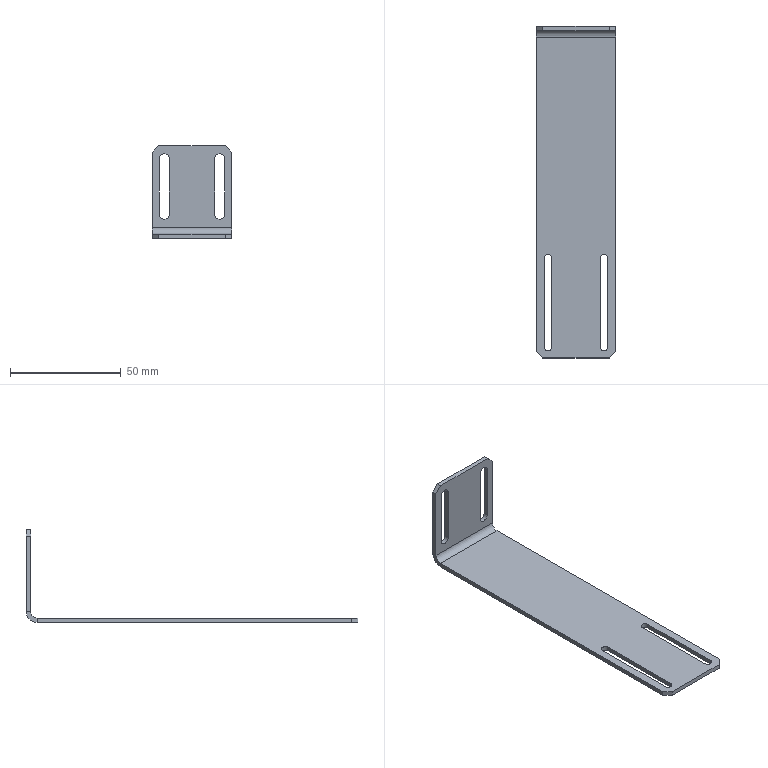Part | NX | 1 solid | 34 faces | box 36 x 150 x 42 mm | volume 12408 mm3 | plane 24 | cylinder 10 | commonest cylinder face diameters 3.5 x4 4.5 x4 6 x1 10 x1
STEP:
#1=CARTESIAN_POINT('',(-18.,70.,-2.));
#2=VERTEX_POINT('',#1);
#3=CARTESIAN_POINT('',(-18.,-72.,-2.));
#4=VERTEX_POINT('',#3);
#5=CARTESIAN_POINT('',(-18.,-75.,-2.));
#6=DIRECTION('',(0.,-1.,0.));
#7=VECTOR('',#6,1000.);
#8=LINE('',#5,#7);
#9=EDGE_CURVE('',#2,#4,#8,.T.);
#10=ORIENTED_EDGE('',*,*,#9,.T.);
#11=CARTESIAN_POINT('',(-18.,-72.,0.));
#12=VERTEX_POINT('',#11);
#13=CARTESIAN_POINT('',(-18.,-72.,-2.));
#14=DIRECTION('',(0.,0.,1.));
#15=VECTOR('',#14,1000.);
#16=LINE('',#13,#15);
#17=EDGE_CURVE('',#4,#12,#16,.T.);
#18=ORIENTED_EDGE('',*,*,#17,.T.);
#19=CARTESIAN_POINT('',(-18.,70.,0.));
#20=VERTEX_POINT('',#19);
#21=CARTESIAN_POINT('',(-18.,-75.,0.));
#22=DIRECTION('',(0.,-1.,0.));
#23=VECTOR('',#22,1000.);
#24=LINE('',#21,#23);
#25=EDGE_CURVE('',#20,#12,#24,.T.);
#26=ORIENTED_EDGE('',*,*,#25,.F.);
#27=CARTESIAN_POINT('',(-18.,70.,0.));
#28=DIRECTION('',(0.,0.,-1.));
#29=VECTOR('',#28,1000.);
#30=LINE('',#27,#29);
#31=EDGE_CURVE('',#20,#2,#30,.T.);
#32=ORIENTED_EDGE('',*,*,#31,.T.);
#33=EDGE_LOOP('',(#10,#18,#26,#32));
#34=FACE_BOUND('',#33,.T.);
#35=CARTESIAN_POINT('',(-18.,-75.,-2.));
#36=DIRECTION('',(-1.,0.,0.));
#37=DIRECTION('',(0.,0.,1.));
#38=AXIS2_PLACEMENT_3D('',#35,#36,#37);
#39=PLANE('',#38);
#40=ADVANCED_FACE('',(#34),#39,.T.);
#41=CARTESIAN_POINT('',(-14.45,-70.,-2.));
#42=VERTEX_POINT('',#41);
#43=CARTESIAN_POINT('',(-10.95,-70.,-2.));
#44=VERTEX_POINT('',#43);
#45=CARTESIAN_POINT('',(-12.7,-70.,-2.));
#46=DIRECTION('',(0.,0.,1.));
#47=DIRECTION('',(1.,0.,0.));
#48=AXIS2_PLACEMENT_3D('',#45,#46,#47);
#49=CIRCLE('',#48,1.75);
#50=EDGE_CURVE('',#42,#44,#49,.T.);
#51=ORIENTED_EDGE('',*,*,#50,.T.);
#52=CARTESIAN_POINT('',(-10.95,-30.,-2.));
#53=VERTEX_POINT('',#52);
#54=CARTESIAN_POINT('',(-10.95,-70.,-2.));
#55=DIRECTION('',(0.,1.,0.));
#56=VECTOR('',#55,1000.);
#57=LINE('',#54,#56);
#58=EDGE_CURVE('',#44,#53,#57,.T.);
#59=ORIENTED_EDGE('',*,*,#58,.T.);
#60=CARTESIAN_POINT('',(-14.45,-30.,-2.));
#61=VERTEX_POINT('',#60);
#62=CARTESIAN_POINT('',(-12.7,-30.,-2.));
#63=DIRECTION('',(0.,0.,1.));
#64=DIRECTION('',(1.,0.,0.));
#65=AXIS2_PLACEMENT_3D('',#62,#63,#64);
#66=CIRCLE('',#65,1.75);
#67=EDGE_CURVE('',#53,#61,#66,.T.);
#68=ORIENTED_EDGE('',*,*,#67,.T.);
#69=CARTESIAN_POINT('',(-14.45,-70.,-2.));
#70=DIRECTION('',(0.,-1.,0.));
#71=VECTOR('',#70,1000.);
#72=LINE('',#69,#71);
#73=EDGE_CURVE('',#61,#42,#72,.T.);
#74=ORIENTED_EDGE('',*,*,#73,.T.);
#75=EDGE_LOOP('',(#51,#59,#68,#74));
#76=FACE_BOUND('',#75,.T.);
#77=CARTESIAN_POINT('',(10.95,-70.,-2.));
#78=VERTEX_POINT('',#77);
#79=CARTESIAN_POINT('',(14.45,-70.,-2.));
#80=VERTEX_POINT('',#79);
#81=CARTESIAN_POINT('',(12.7,-70.,-2.));
#82=DIRECTION('',(0.,0.,1.));
#83=DIRECTION('',(1.,0.,0.));
#84=AXIS2_PLACEMENT_3D('',#81,#82,#83);
#85=CIRCLE('',#84,1.75);
#86=EDGE_CURVE('',#78,#80,#85,.T.);
#87=ORIENTED_EDGE('',*,*,#86,.T.);
#88=CARTESIAN_POINT('',(14.45,-30.,-2.));
#89=VERTEX_POINT('',#88);
#90=CARTESIAN_POINT('',(14.45,-70.,-2.));
#91=DIRECTION('',(0.,1.,0.));
#92=VECTOR('',#91,1000.);
#93=LINE('',#90,#92);
#94=EDGE_CURVE('',#80,#89,#93,.T.);
#95=ORIENTED_EDGE('',*,*,#94,.T.);
#96=CARTESIAN_POINT('',(10.95,-30.,-2.));
#97=VERTEX_POINT('',#96);
#98=CARTESIAN_POINT('',(12.7,-30.,-2.));
#99=DIRECTION('',(0.,0.,1.));
#100=DIRECTION('',(1.,0.,0.));
#101=AXIS2_PLACEMENT_3D('',#98,#99,#100);
#102=CIRCLE('',#101,1.75);
#103=EDGE_CURVE('',#89,#97,#102,.T.);
#104=ORIENTED_EDGE('',*,*,#103,.T.);
#105=CARTESIAN_POINT('',(10.95,-70.,-2.));
#106=DIRECTION('',(0.,-1.,0.));
#107=VECTOR('',#106,1000.);
#108=LINE('',#105,#107);
#109=EDGE_CURVE('',#97,#78,#108,.T.);
#110=ORIENTED_EDGE('',*,*,#109,.T.);
#111=EDGE_LOOP('',(#87,#95,#104,#110));
#112=FACE_BOUND('',#111,.T.);
#113=CARTESIAN_POINT('',(-15.,-75.,-2.));
#114=VERTEX_POINT('',#113);
#115=CARTESIAN_POINT('',(15.,-75.,-2.));
#116=VERTEX_POINT('',#115);
#117=CARTESIAN_POINT('',(-18.,-75.,-2.));
#118=DIRECTION('',(1.,0.,0.));
#119=VECTOR('',#118,1000.);
#120=LINE('',#117,#119);
#121=EDGE_CURVE('',#114,#116,#120,.T.);
#122=ORIENTED_EDGE('',*,*,#121,.F.);
#123=CARTESIAN_POINT('',(-45.,-45.,-2.));
#124=DIRECTION('',(0.7071,-0.7071,0.));
#125=VECTOR('',#124,1000.);
#126=LINE('',#123,#125);
#127=EDGE_CURVE('',#114,#4,#126,.F.);
#128=ORIENTED_EDGE('',*,*,#127,.T.);
#129=ORIENTED_EDGE('',*,*,#9,.F.);
#130=CARTESIAN_POINT('',(18.,70.,-2.));
#131=VERTEX_POINT('',#130);
#132=CARTESIAN_POINT('',(-18.,70.,-2.));
#133=DIRECTION('',(-1.,0.,0.));
#134=VECTOR('',#133,1000.);
#135=LINE('',#132,#134);
#136=EDGE_CURVE('',#2,#131,#135,.F.);
#137=ORIENTED_EDGE('',*,*,#136,.T.);
#138=CARTESIAN_POINT('',(18.,-72.,-2.));
#139=VERTEX_POINT('',#138);
#140=CARTESIAN_POINT('',(18.,-75.,-2.));
#141=DIRECTION('',(0.,1.,0.));
#142=VECTOR('',#141,1000.);
#143=LINE('',#140,#142);
#144=EDGE_CURVE('',#139,#131,#143,.T.);
#145=ORIENTED_EDGE('',*,*,#144,.F.);
#146=CARTESIAN_POINT('',(45.,-45.,-2.));
#147=DIRECTION('',(0.7071,0.7071,0.));
#148=VECTOR('',#147,1000.);
#149=LINE('',#146,#148);
#150=EDGE_CURVE('',#139,#116,#149,.F.);
#151=ORIENTED_EDGE('',*,*,#150,.T.);
#152=EDGE_LOOP('',(#122,#128,#129,#137,#145,#151));
#153=FACE_BOUND('',#152,.T.);
#154=CARTESIAN_POINT('',(0.,0.,-2.));
#155=DIRECTION('',(0.,0.,-1.));
#156=DIRECTION('',(-1.,0.,0.));
#157=AXIS2_PLACEMENT_3D('',#154,#155,#156);
#158=PLANE('',#157);
#159=ADVANCED_FACE('',(#76,#112,#153),#158,.T.);
#160=CARTESIAN_POINT('',(-10.95,-70.,0.));
#161=VERTEX_POINT('',#160);
#162=CARTESIAN_POINT('',(-10.95,-30.,0.));
#163=VERTEX_POINT('',#162);
#164=CARTESIAN_POINT('',(-10.95,-70.,0.));
#165=DIRECTION('',(0.,1.,0.));
#166=VECTOR('',#165,1000.);
#167=LINE('',#164,#166);
#168=EDGE_CURVE('',#161,#163,#167,.T.);
#169=ORIENTED_EDGE('',*,*,#168,.F.);
#170=CARTESIAN_POINT('',(-14.45,-70.,0.));
#171=VERTEX_POINT('',#170);
#172=CARTESIAN_POINT('',(-12.7,-70.,0.));
#173=DIRECTION('',(0.,0.,1.));
#174=DIRECTION('',(1.,0.,0.));
#175=AXIS2_PLACEMENT_3D('',#172,#173,#174);
#176=CIRCLE('',#175,1.75);
#177=EDGE_CURVE('',#171,#161,#176,.T.);
#178=ORIENTED_EDGE('',*,*,#177,.F.);
#179=CARTESIAN_POINT('',(-14.45,-30.,0.));
#180=VERTEX_POINT('',#179);
#181=CARTESIAN_POINT('',(-14.45,-70.,0.));
#182=DIRECTION('',(0.,-1.,0.));
#183=VECTOR('',#182,1000.);
#184=LINE('',#181,#183);
#185=EDGE_CURVE('',#180,#171,#184,.T.);
#186=ORIENTED_EDGE('',*,*,#185,.F.);
#187=CARTESIAN_POINT('',(-12.7,-30.,0.));
#188=DIRECTION('',(0.,0.,1.));
#189=DIRECTION('',(1.,0.,0.));
#190=AXIS2_PLACEMENT_3D('',#187,#188,#189);
#191=CIRCLE('',#190,1.75);
#192=EDGE_CURVE('',#163,#180,#191,.T.);
#193=ORIENTED_EDGE('',*,*,#192,.F.);
#194=EDGE_LOOP('',(#169,#178,#186,#193));
#195=FACE_BOUND('',#194,.T.);
#196=CARTESIAN_POINT('',(14.45,-70.,0.));
#197=VERTEX_POINT('',#196);
#198=CARTESIAN_POINT('',(14.45,-30.,0.));
#199=VERTEX_POINT('',#198);
#200=CARTESIAN_POINT('',(14.45,-70.,0.));
#201=DIRECTION('',(0.,1.,0.));
#202=VECTOR('',#201,1000.);
#203=LINE('',#200,#202);
#204=EDGE_CURVE('',#197,#199,#203,.T.);
#205=ORIENTED_EDGE('',*,*,#204,.F.);
#206=CARTESIAN_POINT('',(10.95,-70.,0.));
#207=VERTEX_POINT('',#206);
#208=CARTESIAN_POINT('',(12.7,-70.,0.));
#209=DIRECTION('',(0.,0.,1.));
#210=DIRECTION('',(1.,0.,0.));
#211=AXIS2_PLACEMENT_3D('',#208,#209,#210);
#212=CIRCLE('',#211,1.75);
#213=EDGE_CURVE('',#207,#197,#212,.T.);
#214=ORIENTED_EDGE('',*,*,#213,.F.);
#215=CARTESIAN_POINT('',(10.95,-30.,0.));
#216=VERTEX_POINT('',#215);
#217=CARTESIAN_POINT('',(10.95,-70.,0.));
#218=DIRECTION('',(0.,-1.,0.));
#219=VECTOR('',#218,1000.);
#220=LINE('',#217,#219);
#221=EDGE_CURVE('',#216,#207,#220,.T.);
#222=ORIENTED_EDGE('',*,*,#221,.F.);
#223=CARTESIAN_POINT('',(12.7,-30.,0.));
#224=DIRECTION('',(0.,0.,1.));
#225=DIRECTION('',(1.,0.,0.));
#226=AXIS2_PLACEMENT_3D('',#223,#224,#225);
#227=CIRCLE('',#226,1.75);
#228=EDGE_CURVE('',#199,#216,#227,.T.);
#229=ORIENTED_EDGE('',*,*,#228,.F.);
#230=EDGE_LOOP('',(#205,#214,#222,#229));
#231=FACE_BOUND('',#230,.T.);
#232=ORIENTED_EDGE('',*,*,#25,.T.);
#233=CARTESIAN_POINT('',(-15.,-75.,0.));
#234=VERTEX_POINT('',#233);
#235=CARTESIAN_POINT('',(-18.,-72.,0.));
#236=DIRECTION('',(-0.7071,0.7071,0.));
#237=VECTOR('',#236,1000.);
#238=LINE('',#235,#237);
#239=EDGE_CURVE('',#12,#234,#238,.F.);
#240=ORIENTED_EDGE('',*,*,#239,.T.);
#241=CARTESIAN_POINT('',(15.,-75.,0.));
#242=VERTEX_POINT('',#241);
#243=CARTESIAN_POINT('',(-18.,-75.,0.));
#244=DIRECTION('',(1.,0.,0.));
#245=VECTOR('',#244,1000.);
#246=LINE('',#243,#245);
#247=EDGE_CURVE('',#234,#242,#246,.T.);
#248=ORIENTED_EDGE('',*,*,#247,.T.);
#249=CARTESIAN_POINT('',(18.,-72.,0.));
#250=VERTEX_POINT('',#249);
#251=CARTESIAN_POINT('',(15.,-75.,0.));
#252=DIRECTION('',(-0.7071,-0.7071,0.));
#253=VECTOR('',#252,1000.);
#254=LINE('',#251,#253);
#255=EDGE_CURVE('',#242,#250,#254,.F.);
#256=ORIENTED_EDGE('',*,*,#255,.T.);
#257=CARTESIAN_POINT('',(18.,70.,0.));
#258=VERTEX_POINT('',#257);
#259=CARTESIAN_POINT('',(18.,-75.,0.));
#260=DIRECTION('',(0.,1.,0.));
#261=VECTOR('',#260,1000.);
#262=LINE('',#259,#261);
#263=EDGE_CURVE('',#250,#258,#262,.T.);
#264=ORIENTED_EDGE('',*,*,#263,.T.);
#265=CARTESIAN_POINT('',(-18.,70.,0.));
#266=DIRECTION('',(-1.,0.,0.));
#267=VECTOR('',#266,1000.);
#268=LINE('',#265,#267);
#269=EDGE_CURVE('',#20,#258,#268,.F.);
#270=ORIENTED_EDGE('',*,*,#269,.F.);
#271=EDGE_LOOP('',(#232,#240,#248,#256,#264,#270));
#272=FACE_BOUND('',#271,.T.);
#273=CARTESIAN_POINT('',(0.,0.,0.));
#274=DIRECTION('',(0.,0.,-1.));
#275=DIRECTION('',(-1.,0.,0.));
#276=AXIS2_PLACEMENT_3D('',#273,#274,#275);
#277=PLANE('',#276);
#278=ADVANCED_FACE('',(#195,#231,#272),#277,.F.);
#279=ORIENTED_EDGE('',*,*,#263,.F.);
#280=CARTESIAN_POINT('',(18.,-72.,-2.));
#281=DIRECTION('',(0.,0.,-1.));
#282=VECTOR('',#281,1000.);
#283=LINE('',#280,#282);
#284=EDGE_CURVE('',#250,#139,#283,.T.);
#285=ORIENTED_EDGE('',*,*,#284,.T.);
#286=ORIENTED_EDGE('',*,*,#144,.T.);
#287=CARTESIAN_POINT('',(18.,70.,0.));
#288=DIRECTION('',(0.,0.,-1.));
#289=VECTOR('',#288,1000.);
#290=LINE('',#287,#289);
#291=EDGE_CURVE('',#258,#131,#290,.T.);
#292=ORIENTED_EDGE('',*,*,#291,.F.);
#293=EDGE_LOOP('',(#279,#285,#286,#292));
#294=FACE_BOUND('',#293,.T.);
#295=CARTESIAN_POINT('',(18.,-75.,-2.));
#296=DIRECTION('',(1.,0.,0.));
#297=DIRECTION('',(0.,0.,-1.));
#298=AXIS2_PLACEMENT_3D('',#295,#296,#297);
#299=PLANE('',#298);
#300=ADVANCED_FACE('',(#294),#299,.T.);
#301=ORIENTED_EDGE('',*,*,#247,.F.);
#302=CARTESIAN_POINT('',(-15.,-75.,-2.));
#303=DIRECTION('',(0.,0.,-1.));
#304=VECTOR('',#303,1000.);
#305=LINE('',#302,#304);
#306=EDGE_CURVE('',#234,#114,#305,.T.);
#307=ORIENTED_EDGE('',*,*,#306,.T.);
#308=ORIENTED_EDGE('',*,*,#121,.T.);
#309=CARTESIAN_POINT('',(15.,-75.,-2.));
#310=DIRECTION('',(0.,0.,1.));
#311=VECTOR('',#310,1000.);
#312=LINE('',#309,#311);
#313=EDGE_CURVE('',#116,#242,#312,.T.);
#314=ORIENTED_EDGE('',*,*,#313,.T.);
#315=EDGE_LOOP('',(#301,#307,#308,#314));
#316=FACE_BOUND('',#315,.T.);
#317=CARTESIAN_POINT('',(-18.,-75.,-2.));
#318=DIRECTION('',(0.,-1.,0.));
#319=DIRECTION('',(0.,0.,-1.));
#320=AXIS2_PLACEMENT_3D('',#317,#318,#319);
#321=PLANE('',#320);
#322=ADVANCED_FACE('',(#316),#321,.T.);
#323=CARTESIAN_POINT('',(18.,73.,3.));
#324=VERTEX_POINT('',#323);
#325=CARTESIAN_POINT('',(18.,75.,3.));
#326=VERTEX_POINT('',#325);
#327=CARTESIAN_POINT('',(18.,75.,3.));
#328=DIRECTION('',(0.,-1.,0.));
#329=VECTOR('',#328,1000.);
#330=LINE('',#327,#329);
#331=EDGE_CURVE('',#324,#326,#330,.F.);
#332=ORIENTED_EDGE('',*,*,#331,.F.);
#333=CARTESIAN_POINT('',(18.,70.,3.));
#334=DIRECTION('',(-1.,0.,0.));
#335=DIRECTION('',(0.,0.,1.));
#336=AXIS2_PLACEMENT_3D('',#333,#334,#335);
#337=CIRCLE('',#336,3.);
#338=EDGE_CURVE('',#258,#324,#337,.F.);
#339=ORIENTED_EDGE('',*,*,#338,.F.);
#340=ORIENTED_EDGE('',*,*,#291,.T.);
#341=CARTESIAN_POINT('',(18.,70.,3.));
#342=DIRECTION('',(-1.,0.,0.));
#343=DIRECTION('',(0.,0.,1.));
#344=AXIS2_PLACEMENT_3D('',#341,#342,#343);
#345=CIRCLE('',#344,5.);
#346=EDGE_CURVE('',#131,#326,#345,.F.);
#347=ORIENTED_EDGE('',*,*,#346,.T.);
#348=EDGE_LOOP('',(#332,#339,#340,#347));
#349=FACE_BOUND('',#348,.T.);
#350=CARTESIAN_POINT('',(18.,70.,3.));
#351=DIRECTION('',(1.,0.,0.));
#352=DIRECTION('',(0.,0.,-1.));
#353=AXIS2_PLACEMENT_3D('',#350,#351,#352);
#354=PLANE('',#353);
#355=ADVANCED_FACE('',(#349),#354,.T.);
#356=CARTESIAN_POINT('',(-18.,73.,3.));
#357=VERTEX_POINT('',#356);
#358=CARTESIAN_POINT('',(-18.,70.,3.));
#359=DIRECTION('',(-1.,0.,0.));
#360=DIRECTION('',(0.,0.,1.));
#361=AXIS2_PLACEMENT_3D('',#358,#359,#360);
#362=CIRCLE('',#361,3.);
#363=EDGE_CURVE('',#357,#20,#362,.T.);
#364=ORIENTED_EDGE('',*,*,#363,.F.);
#365=CARTESIAN_POINT('',(-18.,75.,3.));
#366=VERTEX_POINT('',#365);
#367=CARTESIAN_POINT('',(-18.,73.,3.));
#368=DIRECTION('',(0.,-1.,0.));
#369=VECTOR('',#368,1000.);
#370=LINE('',#367,#369);
#371=EDGE_CURVE('',#357,#366,#370,.F.);
#372=ORIENTED_EDGE('',*,*,#371,.T.);
#373=CARTESIAN_POINT('',(-18.,70.,3.));
#374=DIRECTION('',(-1.,0.,0.));
#375=DIRECTION('',(0.,0.,1.));
#376=AXIS2_PLACEMENT_3D('',#373,#374,#375);
#377=CIRCLE('',#376,5.);
#378=EDGE_CURVE('',#366,#2,#377,.T.);
#379=ORIENTED_EDGE('',*,*,#378,.T.);
#380=ORIENTED_EDGE('',*,*,#31,.F.);
#381=EDGE_LOOP('',(#364,#372,#379,#380));
#382=FACE_BOUND('',#381,.T.);
#383=CARTESIAN_POINT('',(-18.,70.,3.));
#384=DIRECTION('',(1.,0.,0.));
#385=DIRECTION('',(0.,0.,-1.));
#386=AXIS2_PLACEMENT_3D('',#383,#384,#385);
#387=PLANE('',#386);
#388=ADVANCED_FACE('',(#382),#387,.F.);
#389=ORIENTED_EDGE('',*,*,#136,.F.);
#390=ORIENTED_EDGE('',*,*,#378,.F.);
#391=CARTESIAN_POINT('',(18.,75.,3.));
#392=DIRECTION('',(-1.,0.,0.));
#393=VECTOR('',#392,1000.);
#394=LINE('',#391,#393);
#395=EDGE_CURVE('',#366,#326,#394,.F.);
#396=ORIENTED_EDGE('',*,*,#395,.T.);
#397=ORIENTED_EDGE('',*,*,#346,.F.);
#398=EDGE_LOOP('',(#389,#390,#396,#397));
#399=FACE_BOUND('',#398,.T.);
#400=CARTESIAN_POINT('',(-18.,70.,3.));
#401=DIRECTION('',(-1.,0.,0.));
#402=DIRECTION('',(0.,1.,0.));
#403=AXIS2_PLACEMENT_3D('',#400,#401,#402);
#404=CYLINDRICAL_SURFACE('',#403,5.);
#405=ADVANCED_FACE('',(#399),#404,.T.);
#406=ORIENTED_EDGE('',*,*,#269,.T.);
#407=ORIENTED_EDGE('',*,*,#338,.T.);
#408=CARTESIAN_POINT('',(18.,73.,3.));
#409=DIRECTION('',(-1.,0.,0.));
#410=VECTOR('',#409,1000.);
#411=LINE('',#408,#410);
#412=EDGE_CURVE('',#324,#357,#411,.T.);
#413=ORIENTED_EDGE('',*,*,#412,.T.);
#414=ORIENTED_EDGE('',*,*,#363,.T.);
#415=EDGE_LOOP('',(#406,#407,#413,#414));
#416=FACE_BOUND('',#415,.T.);
#417=CARTESIAN_POINT('',(-18.,70.,3.));
#418=DIRECTION('',(-1.,0.,0.));
#419=DIRECTION('',(0.,1.,0.));
#420=AXIS2_PLACEMENT_3D('',#417,#418,#419);
#421=CYLINDRICAL_SURFACE('',#420,3.);
#422=ADVANCED_FACE('',(#416),#421,.F.);
#423=CARTESIAN_POINT('',(18.,75.,37.));
#424=VERTEX_POINT('',#423);
#425=CARTESIAN_POINT('',(18.,75.,0.));
#426=DIRECTION('',(0.,0.,-1.));
#427=VECTOR('',#426,1000.);
#428=LINE('',#425,#427);
#429=EDGE_CURVE('',#424,#326,#428,.T.);
#430=ORIENTED_EDGE('',*,*,#429,.F.);
#431=CARTESIAN_POINT('',(18.,73.,37.));
#432=VERTEX_POINT('',#431);
#433=CARTESIAN_POINT('',(18.,75.,37.));
#434=DIRECTION('',(0.,-1.,0.));
#435=VECTOR('',#434,1000.);
#436=LINE('',#433,#435);
#437=EDGE_CURVE('',#424,#432,#436,.T.);
#438=ORIENTED_EDGE('',*,*,#437,.T.);
#439=CARTESIAN_POINT('',(18.,73.,0.));
#440=DIRECTION('',(0.,0.,1.));
#441=VECTOR('',#440,1000.);
#442=LINE('',#439,#441);
#443=EDGE_CURVE('',#432,#324,#442,.F.);
#444=ORIENTED_EDGE('',*,*,#443,.T.);
#445=ORIENTED_EDGE('',*,*,#331,.T.);
#446=EDGE_LOOP('',(#430,#438,#444,#445));
#447=FACE_BOUND('',#446,.T.);
#448=CARTESIAN_POINT('',(18.,75.,0.));
#449=DIRECTION('',(-1.,0.,0.));
#450=DIRECTION('',(0.,0.,1.));
#451=AXIS2_PLACEMENT_3D('',#448,#449,#450);
#452=PLANE('',#451);
#453=ADVANCED_FACE('',(#447),#452,.F.);
#454=CARTESIAN_POINT('',(-18.,73.,37.));
#455=VERTEX_POINT('',#454);
#456=CARTESIAN_POINT('',(-18.,73.,40.));
#457=DIRECTION('',(0.,0.,-1.));
#458=VECTOR('',#457,1000.);
#459=LINE('',#456,#458);
#460=EDGE_CURVE('',#357,#455,#459,.F.);
#461=ORIENTED_EDGE('',*,*,#460,.T.);
#462=CARTESIAN_POINT('',(-18.,75.,37.));
#463=VERTEX_POINT('',#462);
#464=CARTESIAN_POINT('',(-18.,75.,37.));
#465=DIRECTION('',(0.,1.,0.));
#466=VECTOR('',#465,1000.);
#467=LINE('',#464,#466);
#468=EDGE_CURVE('',#455,#463,#467,.T.);
#469=ORIENTED_EDGE('',*,*,#468,.T.);
#470=CARTESIAN_POINT('',(-18.,75.,0.));
#471=DIRECTION('',(0.,0.,1.));
#472=VECTOR('',#471,1000.);
#473=LINE('',#470,#472);
#474=EDGE_CURVE('',#366,#463,#473,.T.);
#475=ORIENTED_EDGE('',*,*,#474,.F.);
#476=ORIENTED_EDGE('',*,*,#371,.F.);
#477=EDGE_LOOP('',(#461,#469,#475,#476));
#478=FACE_BOUND('',#477,.T.);
#479=CARTESIAN_POINT('',(-18.,75.,40.));
#480=DIRECTION('',(1.,0.,0.));
#481=DIRECTION('',(0.,0.,-1.));
#482=AXIS2_PLACEMENT_3D('',#479,#480,#481);
#483=PLANE('',#482);
#484=ADVANCED_FACE('',(#478),#483,.F.);
#485=CARTESIAN_POINT('',(14.75,75.,9.));
#486=VERTEX_POINT('',#485);
#487=CARTESIAN_POINT('',(14.75,75.,34.));
#488=VERTEX_POINT('',#487);
#489=CARTESIAN_POINT('',(14.75,75.,34.));
#490=DIRECTION('',(0.,0.,1.));
#491=VECTOR('',#490,1000.);
#492=LINE('',#489,#491);
#493=EDGE_CURVE('',#486,#488,#492,.T.);
#494=ORIENTED_EDGE('',*,*,#493,.T.);
#495=CARTESIAN_POINT('',(10.25,75.,34.));
#496=VERTEX_POINT('',#495);
#497=CARTESIAN_POINT('',(12.5,75.,34.));
#498=DIRECTION('',(0.,-1.,0.));
#499=DIRECTION('',(0.,0.,-1.));
#500=AXIS2_PLACEMENT_3D('',#497,#498,#499);
#501=CIRCLE('',#500,2.25);
#502=EDGE_CURVE('',#488,#496,#501,.T.);
#503=ORIENTED_EDGE('',*,*,#502,.T.);
#504=CARTESIAN_POINT('',(10.25,75.,9.));
#505=VERTEX_POINT('',#504);
#506=CARTESIAN_POINT('',(10.25,75.,34.));
#507=DIRECTION('',(0.,0.,-1.));
#508=VECTOR('',#507,1000.);
#509=LINE('',#506,#508);
#510=EDGE_CURVE('',#496,#505,#509,.T.);
#511=ORIENTED_EDGE('',*,*,#510,.T.);
#512=CARTESIAN_POINT('',(12.5,75.,9.));
#513=DIRECTION('',(0.,-1.,0.));
#514=DIRECTION('',(0.,0.,-1.));
#515=AXIS2_PLACEMENT_3D('',#512,#513,#514);
#516=CIRCLE('',#515,2.25);
#517=EDGE_CURVE('',#505,#486,#516,.T.);
#518=ORIENTED_EDGE('',*,*,#517,.T.);
#519=EDGE_LOOP('',(#494,#503,#511,#518));
#520=FACE_BOUND('',#519,.T.);
#521=CARTESIAN_POINT('',(-10.25,75.,9.));
#522=VERTEX_POINT('',#521);
#523=CARTESIAN_POINT('',(-10.25,75.,34.));
#524=VERTEX_POINT('',#523);
#525=CARTESIAN_POINT('',(-10.25,75.,34.));
#526=DIRECTION('',(0.,0.,1.));
#527=VECTOR('',#526,1000.);
#528=LINE('',#525,#527);
#529=EDGE_CURVE('',#522,#524,#528,.T.);
#530=ORIENTED_EDGE('',*,*,#529,.T.);
#531=CARTESIAN_POINT('',(-14.75,75.,34.));
#532=VERTEX_POINT('',#531);
#533=CARTESIAN_POINT('',(-12.5,75.,34.));
#534=DIRECTION('',(0.,-1.,0.));
#535=DIRECTION('',(0.,0.,-1.));
#536=AXIS2_PLACEMENT_3D('',#533,#534,#535);
#537=CIRCLE('',#536,2.25);
#538=EDGE_CURVE('',#524,#532,#537,.T.);
#539=ORIENTED_EDGE('',*,*,#538,.T.);
#540=CARTESIAN_POINT('',(-14.75,75.,9.));
#541=VERTEX_POINT('',#540);
#542=CARTESIAN_POINT('',(-14.75,75.,34.));
#543=DIRECTION('',(0.,0.,-1.));
#544=VECTOR('',#543,1000.);
#545=LINE('',#542,#544);
#546=EDGE_CURVE('',#532,#541,#545,.T.);
#547=ORIENTED_EDGE('',*,*,#546,.T.);
#548=CARTESIAN_POINT('',(-12.5,75.,9.));
#549=DIRECTION('',(0.,-1.,0.));
#550=DIRECTION('',(0.,0.,-1.));
#551=AXIS2_PLACEMENT_3D('',#548,#549,#550);
#552=CIRCLE('',#551,2.25);
#553=EDGE_CURVE('',#541,#522,#552,.T.);
#554=ORIENTED_EDGE('',*,*,#553,.T.);
#555=EDGE_LOOP('',(#530,#539,#547,#554));
#556=FACE_BOUND('',#555,.T.);
#557=CARTESIAN_POINT('',(-15.,75.,40.));
#558=VERTEX_POINT('',#557);
#559=CARTESIAN_POINT('',(15.,75.,40.));
#560=VERTEX_POINT('',#559);
#561=CARTESIAN_POINT('',(0.,75.,40.));
#562=DIRECTION('',(1.,0.,0.));
#563=VECTOR('',#562,1000.);
#564=LINE('',#561,#563);
#565=EDGE_CURVE('',#558,#560,#564,.T.);
#566=ORIENTED_EDGE('',*,*,#565,.T.);
#567=CARTESIAN_POINT('',(18.,75.,37.));
#568=DIRECTION('',(-0.7071,0.,0.7071));
#569=VECTOR('',#568,1000.);
#570=LINE('',#567,#569);
#571=EDGE_CURVE('',#560,#424,#570,.F.);
#572=ORIENTED_EDGE('',*,*,#571,.T.);
#573=ORIENTED_EDGE('',*,*,#429,.T.);
#574=ORIENTED_EDGE('',*,*,#395,.F.);
#575=ORIENTED_EDGE('',*,*,#474,.T.);
#576=CARTESIAN_POINT('',(-15.,75.,40.));
#577=DIRECTION('',(-0.7071,0.,-0.7071));
#578=VECTOR('',#577,1000.);
#579=LINE('',#576,#578);
#580=EDGE_CURVE('',#463,#558,#579,.F.);
#581=ORIENTED_EDGE('',*,*,#580,.T.);
#582=EDGE_LOOP('',(#566,#572,#573,#574,#575,#581));
#583=FACE_BOUND('',#582,.T.);
#584=CARTESIAN_POINT('',(0.,75.,0.));
#585=DIRECTION('',(0.,-1.,0.));
#586=DIRECTION('',(0.,0.,-1.));
#587=AXIS2_PLACEMENT_3D('',#584,#585,#586);
#588=PLANE('',#587);
#589=ADVANCED_FACE('',(#520,#556,#583),#588,.F.);
#590=CARTESIAN_POINT('',(14.75,73.,34.));
#591=VERTEX_POINT('',#590);
#592=CARTESIAN_POINT('',(10.25,73.,34.));
#593=VERTEX_POINT('',#592);
#594=CARTESIAN_POINT('',(12.5,73.,34.));
#595=DIRECTION('',(0.,-1.,0.));
#596=DIRECTION('',(0.,0.,-1.));
#597=AXIS2_PLACEMENT_3D('',#594,#595,#596);
#598=CIRCLE('',#597,2.25);
#599=EDGE_CURVE('',#591,#593,#598,.T.);
#600=ORIENTED_EDGE('',*,*,#599,.F.);
#601=CARTESIAN_POINT('',(14.75,73.,9.));
#602=VERTEX_POINT('',#601);
#603=CARTESIAN_POINT('',(14.75,73.,34.));
#604=DIRECTION('',(0.,0.,1.));
#605=VECTOR('',#604,1000.);
#606=LINE('',#603,#605);
#607=EDGE_CURVE('',#602,#591,#606,.T.);
#608=ORIENTED_EDGE('',*,*,#607,.F.);
#609=CARTESIAN_POINT('',(10.25,73.,9.));
#610=VERTEX_POINT('',#609);
#611=CARTESIAN_POINT('',(12.5,73.,9.));
#612=DIRECTION('',(0.,-1.,0.));
#613=DIRECTION('',(0.,0.,-1.));
#614=AXIS2_PLACEMENT_3D('',#611,#612,#613);
#615=CIRCLE('',#614,2.25);
#616=EDGE_CURVE('',#610,#602,#615,.T.);
#617=ORIENTED_EDGE('',*,*,#616,.F.);
#618=CARTESIAN_POINT('',(10.25,73.,34.));
#619=DIRECTION('',(0.,0.,-1.));
#620=VECTOR('',#619,1000.);
#621=LINE('',#618,#620);
#622=EDGE_CURVE('',#593,#610,#621,.T.);
#623=ORIENTED_EDGE('',*,*,#622,.F.);
#624=EDGE_LOOP('',(#600,#608,#617,#623));
#625=FACE_BOUND('',#624,.T.);
#626=CARTESIAN_POINT('',(-10.25,73.,34.));
#627=VERTEX_POINT('',#626);
#628=CARTESIAN_POINT('',(-14.75,73.,34.));
#629=VERTEX_POINT('',#628);
#630=CARTESIAN_POINT('',(-12.5,73.,34.));
#631=DIRECTION('',(0.,-1.,0.));
#632=DIRECTION('',(0.,0.,-1.));
#633=AXIS2_PLACEMENT_3D('',#630,#631,#632);
#634=CIRCLE('',#633,2.25);
#635=EDGE_CURVE('',#627,#629,#634,.T.);
#636=ORIENTED_EDGE('',*,*,#635,.F.);
#637=CARTESIAN_POINT('',(-10.25,73.,9.));
#638=VERTEX_POINT('',#637);
#639=CARTESIAN_POINT('',(-10.25,73.,34.));
#640=DIRECTION('',(0.,0.,1.));
#641=VECTOR('',#640,1000.);
#642=LINE('',#639,#641);
#643=EDGE_CURVE('',#638,#627,#642,.T.);
#644=ORIENTED_EDGE('',*,*,#643,.F.);
#645=CARTESIAN_POINT('',(-14.75,73.,9.));
#646=VERTEX_POINT('',#645);
#647=CARTESIAN_POINT('',(-12.5,73.,9.));
#648=DIRECTION('',(0.,-1.,0.));
#649=DIRECTION('',(0.,0.,-1.));
#650=AXIS2_PLACEMENT_3D('',#647,#648,#649);
#651=CIRCLE('',#650,2.25);
#652=EDGE_CURVE('',#646,#638,#651,.T.);
#653=ORIENTED_EDGE('',*,*,#652,.F.);
#654=CARTESIAN_POINT('',(-14.75,73.,34.));
#655=DIRECTION('',(0.,0.,-1.));
#656=VECTOR('',#655,1000.);
#657=LINE('',#654,#656);
#658=EDGE_CURVE('',#629,#646,#657,.T.);
#659=ORIENTED_EDGE('',*,*,#658,.F.);
#660=EDGE_LOOP('',(#636,#644,#653,#659));
#661=FACE_BOUND('',#660,.T.);
#662=ORIENTED_EDGE('',*,*,#443,.F.);
#663=CARTESIAN_POINT('',(15.,73.,40.));
#664=VERTEX_POINT('',#663);
#665=CARTESIAN_POINT('',(27.5,73.,27.5));
#666=DIRECTION('',(0.7071,0.,-0.7071));
#667=VECTOR('',#666,1000.);
#668=LINE('',#665,#667);
#669=EDGE_CURVE('',#432,#664,#668,.F.);
#670=ORIENTED_EDGE('',*,*,#669,.T.);
#671=CARTESIAN_POINT('',(-15.,73.,40.));
#672=VERTEX_POINT('',#671);
#673=CARTESIAN_POINT('',(18.,73.,40.));
#674=DIRECTION('',(-1.,0.,0.));
#675=VECTOR('',#674,1000.);
#676=LINE('',#673,#675);
#677=EDGE_CURVE('',#672,#664,#676,.F.);
#678=ORIENTED_EDGE('',*,*,#677,.F.);
#679=CARTESIAN_POINT('',(-27.5,73.,27.5));
#680=DIRECTION('',(0.7071,0.,0.7071));
#681=VECTOR('',#680,1000.);
#682=LINE('',#679,#681);
#683=EDGE_CURVE('',#672,#455,#682,.F.);
#684=ORIENTED_EDGE('',*,*,#683,.T.);
#685=ORIENTED_EDGE('',*,*,#460,.F.);
#686=ORIENTED_EDGE('',*,*,#412,.F.);
#687=EDGE_LOOP('',(#662,#670,#678,#684,#685,#686));
#688=FACE_BOUND('',#687,.T.);
#689=CARTESIAN_POINT('',(0.,73.,0.));
#690=DIRECTION('',(0.,-1.,0.));
#691=DIRECTION('',(0.,0.,-1.));
#692=AXIS2_PLACEMENT_3D('',#689,#690,#691);
#693=PLANE('',#692);
#694=ADVANCED_FACE('',(#625,#661,#688),#693,.T.);
#695=ORIENTED_EDGE('',*,*,#677,.T.);
#696=CARTESIAN_POINT('',(15.,75.,40.));
#697=DIRECTION('',(0.,1.,0.));
#698=VECTOR('',#697,1000.);
#699=LINE('',#696,#698);
#700=EDGE_CURVE('',#664,#560,#699,.T.);
#701=ORIENTED_EDGE('',*,*,#700,.T.);
#702=ORIENTED_EDGE('',*,*,#565,.F.);
#703=CARTESIAN_POINT('',(-15.,75.,40.));
#704=DIRECTION('',(0.,-1.,0.));
#705=VECTOR('',#704,1000.);
#706=LINE('',#703,#705);
#707=EDGE_CURVE('',#558,#672,#706,.T.);
#708=ORIENTED_EDGE('',*,*,#707,.T.);
#709=EDGE_LOOP('',(#695,#701,#702,#708));
#710=FACE_BOUND('',#709,.T.);
#711=CARTESIAN_POINT('',(18.,75.,40.));
#712=DIRECTION('',(0.,0.,-1.));
#713=DIRECTION('',(0.,1.,0.));
#714=AXIS2_PLACEMENT_3D('',#711,#712,#713);
#715=PLANE('',#714);
#716=ADVANCED_FACE('',(#710),#715,.F.);
#717=ORIENTED_EDGE('',*,*,#213,.T.);
#718=CARTESIAN_POINT('',(14.45,-70.,-2.));
#719=DIRECTION('',(0.,0.,1.));
#720=VECTOR('',#719,1000.);
#721=LINE('',#718,#720);
#722=EDGE_CURVE('',#80,#197,#721,.T.);
#723=ORIENTED_EDGE('',*,*,#722,.F.);
#724=ORIENTED_EDGE('',*,*,#86,.F.);
#725=CARTESIAN_POINT('',(10.95,-70.,-2.));
#726=DIRECTION('',(0.,0.,1.));
#727=VECTOR('',#726,1000.);
#728=LINE('',#725,#727);
#729=EDGE_CURVE('',#78,#207,#728,.T.);
#730=ORIENTED_EDGE('',*,*,#729,.T.);
#731=EDGE_LOOP('',(#717,#723,#724,#730));
#732=FACE_BOUND('',#731,.T.);
#733=CARTESIAN_POINT('',(12.7,-70.,-2.));
#734=DIRECTION('',(0.,0.,1.));
#735=DIRECTION('',(1.,0.,0.));
#736=AXIS2_PLACEMENT_3D('',#733,#734,#735);
#737=CYLINDRICAL_SURFACE('',#736,1.75);
#738=ADVANCED_FACE('',(#732),#737,.F.);
#739=ORIENTED_EDGE('',*,*,#221,.T.);
#740=ORIENTED_EDGE('',*,*,#729,.F.);
#741=ORIENTED_EDGE('',*,*,#109,.F.);
#742=CARTESIAN_POINT('',(10.95,-30.,-2.));
#743=DIRECTION('',(0.,0.,1.));
#744=VECTOR('',#743,1000.);
#745=LINE('',#742,#744);
#746=EDGE_CURVE('',#97,#216,#745,.T.);
#747=ORIENTED_EDGE('',*,*,#746,.T.);
#748=EDGE_LOOP('',(#739,#740,#741,#747));
#749=FACE_BOUND('',#748,.T.);
#750=CARTESIAN_POINT('',(10.95,-70.,-2.));
#751=DIRECTION('',(-1.,0.,0.));
#752=DIRECTION('',(0.,0.,1.));
#753=AXIS2_PLACEMENT_3D('',#750,#751,#752);
#754=PLANE('',#753);
#755=ADVANCED_FACE('',(#749),#754,.F.);
#756=ORIENTED_EDGE('',*,*,#228,.T.);
#757=ORIENTED_EDGE('',*,*,#746,.F.);
#758=ORIENTED_EDGE('',*,*,#103,.F.);
#759=CARTESIAN_POINT('',(14.45,-30.,-2.));
#760=DIRECTION('',(0.,0.,1.));
#761=VECTOR('',#760,1000.);
#762=LINE('',#759,#761);
#763=EDGE_CURVE('',#89,#199,#762,.T.);
#764=ORIENTED_EDGE('',*,*,#763,.T.);
#765=EDGE_LOOP('',(#756,#757,#758,#764));
#766=FACE_BOUND('',#765,.T.);
#767=CARTESIAN_POINT('',(12.7,-30.,-2.));
#768=DIRECTION('',(0.,0.,1.));
#769=DIRECTION('',(1.,0.,0.));
#770=AXIS2_PLACEMENT_3D('',#767,#768,#769);
#771=CYLINDRICAL_SURFACE('',#770,1.75);
#772=ADVANCED_FACE('',(#766),#771,.F.);
#773=ORIENTED_EDGE('',*,*,#204,.T.);
#774=ORIENTED_EDGE('',*,*,#763,.F.);
#775=ORIENTED_EDGE('',*,*,#94,.F.);
#776=ORIENTED_EDGE('',*,*,#722,.T.);
#777=EDGE_LOOP('',(#773,#774,#775,#776));
#778=FACE_BOUND('',#777,.T.);
#779=CARTESIAN_POINT('',(14.45,-70.,-2.));
#780=DIRECTION('',(1.,0.,0.));
#781=DIRECTION('',(0.,0.,-1.));
#782=AXIS2_PLACEMENT_3D('',#779,#780,#781);
#783=PLANE('',#782);
#784=ADVANCED_FACE('',(#778),#783,.F.);
#785=ORIENTED_EDGE('',*,*,#177,.T.);
#786=CARTESIAN_POINT('',(-10.95,-70.,-2.));
#787=DIRECTION('',(0.,0.,1.));
#788=VECTOR('',#787,1000.);
#789=LINE('',#786,#788);
#790=EDGE_CURVE('',#44,#161,#789,.T.);
#791=ORIENTED_EDGE('',*,*,#790,.F.);
#792=ORIENTED_EDGE('',*,*,#50,.F.);
#793=CARTESIAN_POINT('',(-14.45,-70.,-2.));
#794=DIRECTION('',(0.,0.,1.));
#795=VECTOR('',#794,1000.);
#796=LINE('',#793,#795);
#797=EDGE_CURVE('',#42,#171,#796,.T.);
#798=ORIENTED_EDGE('',*,*,#797,.T.);
#799=EDGE_LOOP('',(#785,#791,#792,#798));
#800=FACE_BOUND('',#799,.T.);
#801=CARTESIAN_POINT('',(-12.7,-70.,-2.));
#802=DIRECTION('',(0.,0.,1.));
#803=DIRECTION('',(1.,0.,0.));
#804=AXIS2_PLACEMENT_3D('',#801,#802,#803);
#805=CYLINDRICAL_SURFACE('',#804,1.75);
#806=ADVANCED_FACE('',(#800),#805,.F.);
#807=ORIENTED_EDGE('',*,*,#185,.T.);
#808=ORIENTED_EDGE('',*,*,#797,.F.);
#809=ORIENTED_EDGE('',*,*,#73,.F.);
#810=CARTESIAN_POINT('',(-14.45,-30.,-2.));
#811=DIRECTION('',(0.,0.,1.));
#812=VECTOR('',#811,1000.);
#813=LINE('',#810,#812);
#814=EDGE_CURVE('',#61,#180,#813,.T.);
#815=ORIENTED_EDGE('',*,*,#814,.T.);
#816=EDGE_LOOP('',(#807,#808,#809,#815));
#817=FACE_BOUND('',#816,.T.);
#818=CARTESIAN_POINT('',(-14.45,-70.,-2.));
#819=DIRECTION('',(-1.,0.,0.));
#820=DIRECTION('',(0.,-1.,0.));
#821=AXIS2_PLACEMENT_3D('',#818,#819,#820);
#822=PLANE('',#821);
#823=ADVANCED_FACE('',(#817),#822,.F.);
#824=ORIENTED_EDGE('',*,*,#192,.T.);
#825=ORIENTED_EDGE('',*,*,#814,.F.);
#826=ORIENTED_EDGE('',*,*,#67,.F.);
#827=CARTESIAN_POINT('',(-10.95,-30.,-2.));
#828=DIRECTION('',(0.,0.,1.));
#829=VECTOR('',#828,1000.);
#830=LINE('',#827,#829);
#831=EDGE_CURVE('',#53,#163,#830,.T.);
#832=ORIENTED_EDGE('',*,*,#831,.T.);
#833=EDGE_LOOP('',(#824,#825,#826,#832));
#834=FACE_BOUND('',#833,.T.);
#835=CARTESIAN_POINT('',(-12.7,-30.,-2.));
#836=DIRECTION('',(0.,0.,1.));
#837=DIRECTION('',(1.,0.,0.));
#838=AXIS2_PLACEMENT_3D('',#835,#836,#837);
#839=CYLINDRICAL_SURFACE('',#838,1.75);
#840=ADVANCED_FACE('',(#834),#839,.F.);
#841=ORIENTED_EDGE('',*,*,#168,.T.);
#842=ORIENTED_EDGE('',*,*,#831,.F.);
#843=ORIENTED_EDGE('',*,*,#58,.F.);
#844=ORIENTED_EDGE('',*,*,#790,.T.);
#845=EDGE_LOOP('',(#841,#842,#843,#844));
#846=FACE_BOUND('',#845,.T.);
#847=CARTESIAN_POINT('',(-10.95,-70.,-2.));
#848=DIRECTION('',(1.,0.,0.));
#849=DIRECTION('',(0.,1.,0.));
#850=AXIS2_PLACEMENT_3D('',#847,#848,#849);
#851=PLANE('',#850);
#852=ADVANCED_FACE('',(#846),#851,.F.);
#853=ORIENTED_EDGE('',*,*,#635,.T.);
#854=CARTESIAN_POINT('',(-14.75,75.,34.));
#855=DIRECTION('',(0.,-1.,0.));
#856=VECTOR('',#855,1000.);
#857=LINE('',#854,#856);
#858=EDGE_CURVE('',#532,#629,#857,.T.);
#859=ORIENTED_EDGE('',*,*,#858,.F.);
#860=ORIENTED_EDGE('',*,*,#538,.F.);
#861=CARTESIAN_POINT('',(-10.25,75.,34.));
#862=DIRECTION('',(0.,-1.,0.));
#863=VECTOR('',#862,1000.);
#864=LINE('',#861,#863);
#865=EDGE_CURVE('',#524,#627,#864,.T.);
#866=ORIENTED_EDGE('',*,*,#865,.T.);
#867=EDGE_LOOP('',(#853,#859,#860,#866));
#868=FACE_BOUND('',#867,.T.);
#869=CARTESIAN_POINT('',(-12.5,75.,34.));
#870=DIRECTION('',(0.,-1.,0.));
#871=DIRECTION('',(0.,0.,-1.));
#872=AXIS2_PLACEMENT_3D('',#869,#870,#871);
#873=CYLINDRICAL_SURFACE('',#872,2.25);
#874=ADVANCED_FACE('',(#868),#873,.F.);
#875=ORIENTED_EDGE('',*,*,#643,.T.);
#876=ORIENTED_EDGE('',*,*,#865,.F.);
#877=ORIENTED_EDGE('',*,*,#529,.F.);
#878=CARTESIAN_POINT('',(-10.25,75.,9.));
#879=DIRECTION('',(0.,-1.,0.));
#880=VECTOR('',#879,1000.);
#881=LINE('',#878,#880);
#882=EDGE_CURVE('',#522,#638,#881,.T.);
#883=ORIENTED_EDGE('',*,*,#882,.T.);
#884=EDGE_LOOP('',(#875,#876,#877,#883));
#885=FACE_BOUND('',#884,.T.);
#886=CARTESIAN_POINT('',(-10.25,75.,34.));
#887=DIRECTION('',(1.,0.,0.));
#888=DIRECTION('',(0.,0.,-1.));
#889=AXIS2_PLACEMENT_3D('',#886,#887,#888);
#890=PLANE('',#889);
#891=ADVANCED_FACE('',(#885),#890,.F.);
#892=ORIENTED_EDGE('',*,*,#652,.T.);
#893=ORIENTED_EDGE('',*,*,#882,.F.);
#894=ORIENTED_EDGE('',*,*,#553,.F.);
#895=CARTESIAN_POINT('',(-14.75,75.,9.));
#896=DIRECTION('',(0.,-1.,0.));
#897=VECTOR('',#896,1000.);
#898=LINE('',#895,#897);
#899=EDGE_CURVE('',#541,#646,#898,.T.);
#900=ORIENTED_EDGE('',*,*,#899,.T.);
#901=EDGE_LOOP('',(#892,#893,#894,#900));
#902=FACE_BOUND('',#901,.T.);
#903=CARTESIAN_POINT('',(-12.5,75.,9.));
#904=DIRECTION('',(0.,-1.,0.));
#905=DIRECTION('',(0.,0.,-1.));
#906=AXIS2_PLACEMENT_3D('',#903,#904,#905);
#907=CYLINDRICAL_SURFACE('',#906,2.25);
#908=ADVANCED_FACE('',(#902),#907,.F.);
#909=ORIENTED_EDGE('',*,*,#658,.T.);
#910=ORIENTED_EDGE('',*,*,#899,.F.);
#911=ORIENTED_EDGE('',*,*,#546,.F.);
#912=ORIENTED_EDGE('',*,*,#858,.T.);
#913=EDGE_LOOP('',(#909,#910,#911,#912));
#914=FACE_BOUND('',#913,.T.);
#915=CARTESIAN_POINT('',(-14.75,75.,34.));
#916=DIRECTION('',(-1.,0.,0.));
#917=DIRECTION('',(0.,0.,1.));
#918=AXIS2_PLACEMENT_3D('',#915,#916,#917);
#919=PLANE('',#918);
#920=ADVANCED_FACE('',(#914),#919,.F.);
#921=ORIENTED_EDGE('',*,*,#599,.T.);
#922=CARTESIAN_POINT('',(10.25,75.,34.));
#923=DIRECTION('',(0.,-1.,0.));
#924=VECTOR('',#923,1000.);
#925=LINE('',#922,#924);
#926=EDGE_CURVE('',#496,#593,#925,.T.);
#927=ORIENTED_EDGE('',*,*,#926,.F.);
#928=ORIENTED_EDGE('',*,*,#502,.F.);
#929=CARTESIAN_POINT('',(14.75,75.,34.));
#930=DIRECTION('',(0.,-1.,0.));
#931=VECTOR('',#930,1000.);
#932=LINE('',#929,#931);
#933=EDGE_CURVE('',#488,#591,#932,.T.);
#934=ORIENTED_EDGE('',*,*,#933,.T.);
#935=EDGE_LOOP('',(#921,#927,#928,#934));
#936=FACE_BOUND('',#935,.T.);
#937=CARTESIAN_POINT('',(12.5,75.,34.));
#938=DIRECTION('',(0.,-1.,0.));
#939=DIRECTION('',(0.,0.,-1.));
#940=AXIS2_PLACEMENT_3D('',#937,#938,#939);
#941=CYLINDRICAL_SURFACE('',#940,2.25);
#942=ADVANCED_FACE('',(#936),#941,.F.);
#943=ORIENTED_EDGE('',*,*,#607,.T.);
#944=ORIENTED_EDGE('',*,*,#933,.F.);
#945=ORIENTED_EDGE('',*,*,#493,.F.);
#946=CARTESIAN_POINT('',(14.75,75.,9.));
#947=DIRECTION('',(0.,-1.,0.));
#948=VECTOR('',#947,1000.);
#949=LINE('',#946,#948);
#950=EDGE_CURVE('',#486,#602,#949,.T.);
#951=ORIENTED_EDGE('',*,*,#950,.T.);
#952=EDGE_LOOP('',(#943,#944,#945,#951));
#953=FACE_BOUND('',#952,.T.);
#954=CARTESIAN_POINT('',(14.75,75.,34.));
#955=DIRECTION('',(1.,0.,0.));
#956=DIRECTION('',(0.,0.,-1.));
#957=AXIS2_PLACEMENT_3D('',#954,#955,#956);
#958=PLANE('',#957);
#959=ADVANCED_FACE('',(#953),#958,.F.);
#960=ORIENTED_EDGE('',*,*,#616,.T.);
#961=ORIENTED_EDGE('',*,*,#950,.F.);
#962=ORIENTED_EDGE('',*,*,#517,.F.);
#963=CARTESIAN_POINT('',(10.25,75.,9.));
#964=DIRECTION('',(0.,-1.,0.));
#965=VECTOR('',#964,1000.);
#966=LINE('',#963,#965);
#967=EDGE_CURVE('',#505,#610,#966,.T.);
#968=ORIENTED_EDGE('',*,*,#967,.T.);
#969=EDGE_LOOP('',(#960,#961,#962,#968));
#970=FACE_BOUND('',#969,.T.);
#971=CARTESIAN_POINT('',(12.5,75.,9.));
#972=DIRECTION('',(0.,-1.,0.));
#973=DIRECTION('',(0.,0.,-1.));
#974=AXIS2_PLACEMENT_3D('',#971,#972,#973);
#975=CYLINDRICAL_SURFACE('',#974,2.25);
#976=ADVANCED_FACE('',(#970),#975,.F.);
#977=ORIENTED_EDGE('',*,*,#622,.T.);
#978=ORIENTED_EDGE('',*,*,#967,.F.);
#979=ORIENTED_EDGE('',*,*,#510,.F.);
#980=ORIENTED_EDGE('',*,*,#926,.T.);
#981=EDGE_LOOP('',(#977,#978,#979,#980));
#982=FACE_BOUND('',#981,.T.);
#983=CARTESIAN_POINT('',(10.25,75.,34.));
#984=DIRECTION('',(-1.,0.,0.));
#985=DIRECTION('',(0.,0.,1.));
#986=AXIS2_PLACEMENT_3D('',#983,#984,#985);
#987=PLANE('',#986);
#988=ADVANCED_FACE('',(#982),#987,.F.);
#989=ORIENTED_EDGE('',*,*,#127,.F.);
#990=ORIENTED_EDGE('',*,*,#306,.F.);
#991=ORIENTED_EDGE('',*,*,#239,.F.);
#992=ORIENTED_EDGE('',*,*,#17,.F.);
#993=EDGE_LOOP('',(#989,#990,#991,#992));
#994=FACE_BOUND('',#993,.T.);
#995=CARTESIAN_POINT('',(-18.,-72.,-2.));
#996=DIRECTION('',(0.7071,0.7071,0.));
#997=DIRECTION('',(0.,0.,1.));
#998=AXIS2_PLACEMENT_3D('',#995,#996,#997);
#999=PLANE('',#998);
#1000=ADVANCED_FACE('',(#994),#999,.F.);
#1001=ORIENTED_EDGE('',*,*,#150,.F.);
#1002=ORIENTED_EDGE('',*,*,#284,.F.);
#1003=ORIENTED_EDGE('',*,*,#255,.F.);
#1004=ORIENTED_EDGE('',*,*,#313,.F.);
#1005=EDGE_LOOP('',(#1001,#1002,#1003,#1004));
#1006=FACE_BOUND('',#1005,.T.);
#1007=CARTESIAN_POINT('',(15.,-75.,-2.));
#1008=DIRECTION('',(-0.7071,0.7071,0.));
#1009=DIRECTION('',(0.,0.,1.));
#1010=AXIS2_PLACEMENT_3D('',#1007,#1008,#1009);
#1011=PLANE('',#1010);
#1012=ADVANCED_FACE('',(#1006),#1011,.F.);
#1013=ORIENTED_EDGE('',*,*,#571,.F.);
#1014=ORIENTED_EDGE('',*,*,#700,.F.);
#1015=ORIENTED_EDGE('',*,*,#669,.F.);
#1016=ORIENTED_EDGE('',*,*,#437,.F.);
#1017=EDGE_LOOP('',(#1013,#1014,#1015,#1016));
#1018=FACE_BOUND('',#1017,.T.);
#1019=CARTESIAN_POINT('',(18.,75.,37.));
#1020=DIRECTION('',(-0.7071,0.,-0.7071));
#1021=DIRECTION('',(0.,-1.,0.));
#1022=AXIS2_PLACEMENT_3D('',#1019,#1020,#1021);
#1023=PLANE('',#1022);
#1024=ADVANCED_FACE('',(#1018),#1023,.F.);
#1025=ORIENTED_EDGE('',*,*,#580,.F.);
#1026=ORIENTED_EDGE('',*,*,#468,.F.);
#1027=ORIENTED_EDGE('',*,*,#683,.F.);
#1028=ORIENTED_EDGE('',*,*,#707,.F.);
#1029=EDGE_LOOP('',(#1025,#1026,#1027,#1028));
#1030=FACE_BOUND('',#1029,.T.);
#1031=CARTESIAN_POINT('',(-15.,75.,40.));
#1032=DIRECTION('',(0.7071,0.,-0.7071));
#1033=DIRECTION('',(0.,-1.,0.));
#1034=AXIS2_PLACEMENT_3D('',#1031,#1032,#1033);
#1035=PLANE('',#1034);
#1036=ADVANCED_FACE('',(#1030),#1035,.F.);
#1037=CLOSED_SHELL('',(#40,#159,#278,#300,#322,#355,#388,#405,#422,#453,#484,#589,#694,#716,#738,#755,#772,#784,#806,#823,#840,#852,#874,#891,#908,#920,#942,#959,#976,#988,#1000,#1012,#1024,#1036));
#1038=MANIFOLD_SOLID_BREP('',#1037);
#1039=(LENGTH_UNIT()NAMED_UNIT(*)SI_UNIT(.MILLI.,.METRE.));
#1040=UNCERTAINTY_MEASURE_WITH_UNIT(LENGTH_MEASURE(0.00001),#1039,'','');
#1041=(NAMED_UNIT(*)PLANE_ANGLE_UNIT()SI_UNIT($,.RADIAN.));
#1042=(NAMED_UNIT(*)SI_UNIT($,.STERADIAN.)SOLID_ANGLE_UNIT());
#1043=(GEOMETRIC_REPRESENTATION_CONTEXT(3)GLOBAL_UNCERTAINTY_ASSIGNED_CONTEXT((#1040))GLOBAL_UNIT_ASSIGNED_CONTEXT((#1039,#1041,#1042))REPRESENTATION_CONTEXT('',''));
#1044=ADVANCED_BREP_SHAPE_REPRESENTATION('',(#1038),#1043);